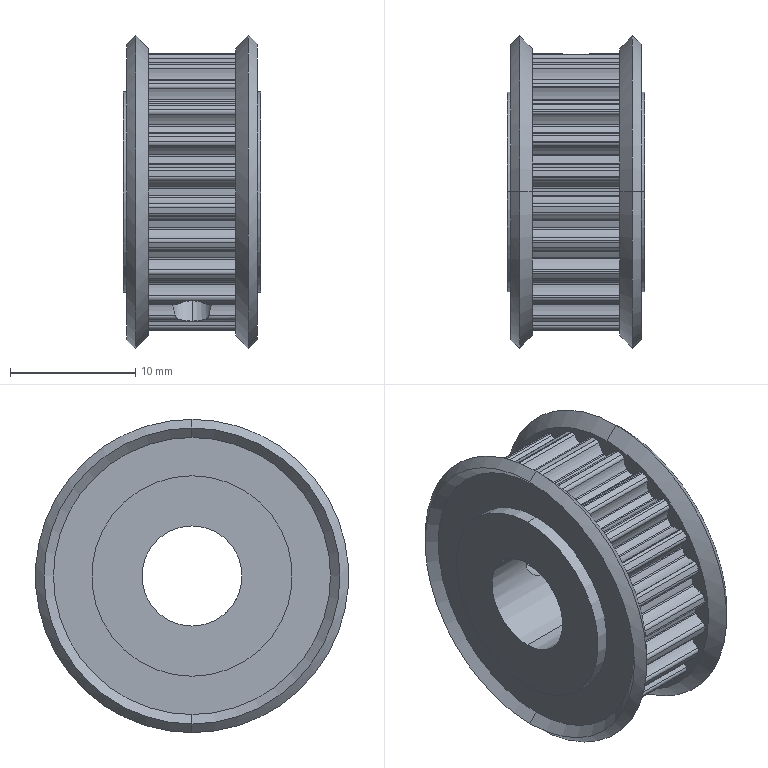Part | STEP file | 11-HTPA24S3M060_A_P8_a11 | 1 solid | 256 faces | box 11 x 25 x 25 mm | volume 3142 mm3 | cylinder 238 | cone 12 | plane 6 | commonest cylinder face diameters 0.56 x62 0.3 x59 3.95 x56 19.94 x27 22.16 x24 3.242 x4